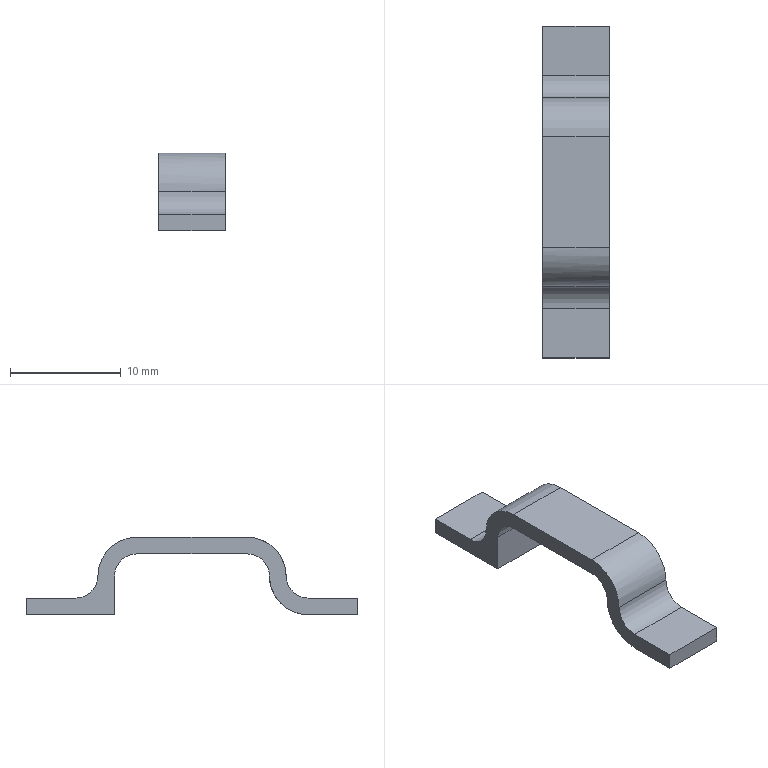Part | NX | features BREP 1 | 1 solid | 18 faces | box 6 x 30 x 7 mm | volume 342.282 mm3 | plane 11 | cylinder 7 | commonest cylinder face diameters 4 x4 7 x3
STEP:
#1=CARTESIAN_POINT('',(41.,114.5,3.5));
#2=VERTEX_POINT('',#1);
#3=CARTESIAN_POINT('',(47.,114.5,3.5));
#4=VERTEX_POINT('',#3);
#5=CARTESIAN_POINT('',(0.,114.5,3.5));
#6=DIRECTION('',(1.,0.,0.));
#7=VECTOR('',#6,1000.);
#8=LINE('',#5,#7);
#9=EDGE_CURVE('',#2,#4,#8,.T.);
#10=ORIENTED_EDGE('',*,*,#9,.F.);
#11=CARTESIAN_POINT('',(41.,111.,7.));
#12=VERTEX_POINT('',#11);
#13=CARTESIAN_POINT('',(41.,111.,3.5));
#14=DIRECTION('',(-1.,0.,0.));
#15=DIRECTION('',(0.,0.,-1.));
#16=AXIS2_PLACEMENT_3D('',#13,#14,#15);
#17=CIRCLE('',#16,3.5);
#18=EDGE_CURVE('',#12,#2,#17,.T.);
#19=ORIENTED_EDGE('',*,*,#18,.F.);
#20=CARTESIAN_POINT('',(47.,111.,7.));
#21=VERTEX_POINT('',#20);
#22=CARTESIAN_POINT('',(0.,111.,7.));
#23=DIRECTION('',(1.,0.,0.));
#24=VECTOR('',#23,1000.);
#25=LINE('',#22,#24);
#26=EDGE_CURVE('',#12,#21,#25,.T.);
#27=ORIENTED_EDGE('',*,*,#26,.T.);
#28=CARTESIAN_POINT('',(47.,111.,3.5));
#29=DIRECTION('',(1.,0.,0.));
#30=DIRECTION('',(0.,0.,-1.));
#31=AXIS2_PLACEMENT_3D('',#28,#29,#30);
#32=CIRCLE('',#31,3.5);
#33=EDGE_CURVE('',#4,#21,#32,.T.);
#34=ORIENTED_EDGE('',*,*,#33,.F.);
#35=EDGE_LOOP('',(#10,#19,#27,#34));
#36=FACE_BOUND('',#35,.T.);
#37=CARTESIAN_POINT('',(0.,111.,3.5));
#38=DIRECTION('',(1.,0.,0.));
#39=DIRECTION('',(0.,1.,0.));
#40=AXIS2_PLACEMENT_3D('',#37,#38,#39);
#41=CYLINDRICAL_SURFACE('',#40,3.5);
#42=ADVANCED_FACE('',(#36),#41,.T.);
#43=ORIENTED_EDGE('',*,*,#9,.T.);
#44=CARTESIAN_POINT('',(47.,116.5,1.5));
#45=VERTEX_POINT('',#44);
#46=CARTESIAN_POINT('',(47.,116.5,3.5));
#47=DIRECTION('',(-1.,0.,0.));
#48=DIRECTION('',(0.,0.,-1.));
#49=AXIS2_PLACEMENT_3D('',#46,#47,#48);
#50=CIRCLE('',#49,2.);
#51=EDGE_CURVE('',#45,#4,#50,.T.);
#52=ORIENTED_EDGE('',*,*,#51,.F.);
#53=CARTESIAN_POINT('',(41.,116.5,1.5));
#54=VERTEX_POINT('',#53);
#55=CARTESIAN_POINT('',(0.,116.5,1.5));
#56=DIRECTION('',(-1.,0.,0.));
#57=VECTOR('',#56,1000.);
#58=LINE('',#55,#57);
#59=EDGE_CURVE('',#45,#54,#58,.T.);
#60=ORIENTED_EDGE('',*,*,#59,.T.);
#61=CARTESIAN_POINT('',(41.,116.5,3.5));
#62=DIRECTION('',(1.,0.,0.));
#63=DIRECTION('',(0.,0.,-1.));
#64=AXIS2_PLACEMENT_3D('',#61,#62,#63);
#65=CIRCLE('',#64,2.);
#66=EDGE_CURVE('',#2,#54,#65,.T.);
#67=ORIENTED_EDGE('',*,*,#66,.F.);
#68=EDGE_LOOP('',(#43,#52,#60,#67));
#69=FACE_BOUND('',#68,.T.);
#70=CARTESIAN_POINT('',(0.,116.5,3.5));
#71=DIRECTION('',(1.,0.,0.));
#72=DIRECTION('',(0.,-1.,0.));
#73=AXIS2_PLACEMENT_3D('',#70,#71,#72);
#74=CYLINDRICAL_SURFACE('',#73,2.);
#75=ADVANCED_FACE('',(#69),#74,.F.);
#76=CARTESIAN_POINT('',(41.,97.5,3.5));
#77=VERTEX_POINT('',#76);
#78=CARTESIAN_POINT('',(41.,101.,7.));
#79=VERTEX_POINT('',#78);
#80=CARTESIAN_POINT('',(41.,97.5,3.5));
#81=CARTESIAN_POINT('',(41.,97.5,3.867));
#82=CARTESIAN_POINT('',(41.,97.548,4.233));
#83=CARTESIAN_POINT('',(41.,97.644,4.591));
#84=CARTESIAN_POINT('',(41.,97.928,5.274));
#85=CARTESIAN_POINT('',(41.,98.377,5.861));
#86=CARTESIAN_POINT('',(41.,98.64,6.124));
#87=CARTESIAN_POINT('',(41.,99.227,6.573));
#88=CARTESIAN_POINT('',(41.,99.909,6.856));
#89=CARTESIAN_POINT('',(41.,100.267,6.952));
#90=CARTESIAN_POINT('',(41.,100.634,7.));
#91=CARTESIAN_POINT('',(41.,101.,7.));
#92=B_SPLINE_CURVE_WITH_KNOTS('',5,(#80,#81,#82,#83,#84,#85,#86,#87,#88,#89,#90,#91),.UNSPECIFIED.,.F.,.F.,(6,3,3,6),(0.,0.3334,0.6668,1.),.UNSPECIFIED.);
#93=EDGE_CURVE('',#77,#79,#92,.T.);
#94=ORIENTED_EDGE('',*,*,#93,.T.);
#95=CARTESIAN_POINT('',(41.,106.,7.));
#96=DIRECTION('',(0.,1.,0.));
#97=VECTOR('',#96,1000.);
#98=LINE('',#95,#97);
#99=EDGE_CURVE('',#79,#12,#98,.T.);
#100=ORIENTED_EDGE('',*,*,#99,.T.);
#101=ORIENTED_EDGE('',*,*,#18,.T.);
#102=ORIENTED_EDGE('',*,*,#66,.T.);
#103=CARTESIAN_POINT('',(41.,121.,1.5));
#104=VERTEX_POINT('',#103);
#105=CARTESIAN_POINT('',(41.,118.75,1.5));
#106=DIRECTION('',(0.,1.,0.));
#107=VECTOR('',#106,1000.);
#108=LINE('',#105,#107);
#109=EDGE_CURVE('',#54,#104,#108,.T.);
#110=ORIENTED_EDGE('',*,*,#109,.T.);
#111=CARTESIAN_POINT('',(41.,121.,0.));
#112=VERTEX_POINT('',#111);
#113=CARTESIAN_POINT('',(41.,121.,0.75));
#114=DIRECTION('',(0.,0.,1.));
#115=VECTOR('',#114,1000.);
#116=LINE('',#113,#115);
#117=EDGE_CURVE('',#112,#104,#116,.T.);
#118=ORIENTED_EDGE('',*,*,#117,.F.);
#119=CARTESIAN_POINT('',(41.,113.,0.));
#120=VERTEX_POINT('',#119);
#121=CARTESIAN_POINT('',(41.,117.,0.));
#122=DIRECTION('',(0.,1.,0.));
#123=VECTOR('',#122,1000.);
#124=LINE('',#121,#123);
#125=EDGE_CURVE('',#120,#112,#124,.T.);
#126=ORIENTED_EDGE('',*,*,#125,.F.);
#127=CARTESIAN_POINT('',(41.,113.,3.5));
#128=VERTEX_POINT('',#127);
#129=CARTESIAN_POINT('',(41.,113.,1.75));
#130=DIRECTION('',(0.,0.,1.));
#131=VECTOR('',#130,1000.);
#132=LINE('',#129,#131);
#133=EDGE_CURVE('',#120,#128,#132,.T.);
#134=ORIENTED_EDGE('',*,*,#133,.T.);
#135=CARTESIAN_POINT('',(41.,111.,5.5));
#136=VERTEX_POINT('',#135);
#137=CARTESIAN_POINT('',(41.,111.,3.5));
#138=DIRECTION('',(1.,0.,0.));
#139=DIRECTION('',(0.,0.,-1.));
#140=AXIS2_PLACEMENT_3D('',#137,#138,#139);
#141=CIRCLE('',#140,2.);
#142=EDGE_CURVE('',#128,#136,#141,.T.);
#143=ORIENTED_EDGE('',*,*,#142,.T.);
#144=CARTESIAN_POINT('',(41.,101.,5.5));
#145=VERTEX_POINT('',#144);
#146=CARTESIAN_POINT('',(41.,106.,5.5));
#147=DIRECTION('',(0.,1.,0.));
#148=VECTOR('',#147,1000.);
#149=LINE('',#146,#148);
#150=EDGE_CURVE('',#145,#136,#149,.T.);
#151=ORIENTED_EDGE('',*,*,#150,.F.);
#152=CARTESIAN_POINT('',(41.,99.,3.5));
#153=VERTEX_POINT('',#152);
#154=CARTESIAN_POINT('',(41.,101.,3.5));
#155=DIRECTION('',(1.,0.,0.));
#156=DIRECTION('',(0.,0.,-1.));
#157=AXIS2_PLACEMENT_3D('',#154,#155,#156);
#158=CIRCLE('',#157,2.);
#159=EDGE_CURVE('',#145,#153,#158,.T.);
#160=ORIENTED_EDGE('',*,*,#159,.T.);
#161=CARTESIAN_POINT('',(41.,95.5,0.));
#162=VERTEX_POINT('',#161);
#163=CARTESIAN_POINT('',(41.,99.,3.5));
#164=CARTESIAN_POINT('',(41.,99.,3.133));
#165=CARTESIAN_POINT('',(41.,98.952,2.767));
#166=CARTESIAN_POINT('',(41.,98.856,2.409));
#167=CARTESIAN_POINT('',(41.,98.572,1.726));
#168=CARTESIAN_POINT('',(41.,98.123,1.139));
#169=CARTESIAN_POINT('',(41.,97.86,0.8765));
#170=CARTESIAN_POINT('',(41.,97.273,0.4271));
#171=CARTESIAN_POINT('',(41.,96.591,0.1438));
#172=CARTESIAN_POINT('',(41.,96.233,0.04793));
#173=CARTESIAN_POINT('',(41.,95.866,0.));
#174=CARTESIAN_POINT('',(41.,95.5,0.));
#175=B_SPLINE_CURVE_WITH_KNOTS('',5,(#163,#164,#165,#166,#167,#168,#169,#170,#171,#172,#173,#174),.UNSPECIFIED.,.F.,.F.,(6,3,3,6),(0.,0.3334,0.6668,1.),.UNSPECIFIED.);
#176=EDGE_CURVE('',#153,#162,#175,.T.);
#177=ORIENTED_EDGE('',*,*,#176,.T.);
#178=CARTESIAN_POINT('',(41.,91.,0.));
#179=VERTEX_POINT('',#178);
#180=CARTESIAN_POINT('',(41.,93.25,0.));
#181=DIRECTION('',(0.,1.,0.));
#182=VECTOR('',#181,1000.);
#183=LINE('',#180,#182);
#184=EDGE_CURVE('',#179,#162,#183,.T.);
#185=ORIENTED_EDGE('',*,*,#184,.F.);
#186=CARTESIAN_POINT('',(41.,91.,1.5));
#187=VERTEX_POINT('',#186);
#188=CARTESIAN_POINT('',(41.,91.,0.75));
#189=DIRECTION('',(0.,0.,1.));
#190=VECTOR('',#189,1000.);
#191=LINE('',#188,#190);
#192=EDGE_CURVE('',#179,#187,#191,.T.);
#193=ORIENTED_EDGE('',*,*,#192,.T.);
#194=CARTESIAN_POINT('',(41.,95.5,1.5));
#195=VERTEX_POINT('',#194);
#196=CARTESIAN_POINT('',(41.,93.25,1.5));
#197=DIRECTION('',(0.,1.,0.));
#198=VECTOR('',#197,1000.);
#199=LINE('',#196,#198);
#200=EDGE_CURVE('',#187,#195,#199,.T.);
#201=ORIENTED_EDGE('',*,*,#200,.T.);
#202=CARTESIAN_POINT('',(41.,95.5,3.5));
#203=DIRECTION('',(1.,0.,0.));
#204=DIRECTION('',(0.,0.,-1.));
#205=AXIS2_PLACEMENT_3D('',#202,#203,#204);
#206=CIRCLE('',#205,2.);
#207=EDGE_CURVE('',#195,#77,#206,.T.);
#208=ORIENTED_EDGE('',*,*,#207,.T.);
#209=EDGE_LOOP('',(#94,#100,#101,#102,#110,#118,#126,#134,#143,#151,#160,#177,#185,#193,#201,#208));
#210=FACE_BOUND('',#209,.T.);
#211=CARTESIAN_POINT('',(41.,121.,1.5));
#212=DIRECTION('',(1.,0.,0.));
#213=DIRECTION('',(0.,-1.,0.));
#214=AXIS2_PLACEMENT_3D('',#211,#212,#213);
#215=PLANE('',#214);
#216=ADVANCED_FACE('',(#210),#215,.F.);
#217=CARTESIAN_POINT('',(47.,101.,7.));
#218=VERTEX_POINT('',#217);
#219=CARTESIAN_POINT('',(44.,101.,7.));
#220=DIRECTION('',(-1.,0.,0.));
#221=VECTOR('',#220,1000.);
#222=LINE('',#219,#221);
#223=EDGE_CURVE('',#218,#79,#222,.T.);
#224=ORIENTED_EDGE('',*,*,#223,.F.);
#225=CARTESIAN_POINT('',(47.,106.,7.));
#226=DIRECTION('',(0.,-1.,0.));
#227=VECTOR('',#226,1000.);
#228=LINE('',#225,#227);
#229=EDGE_CURVE('',#21,#218,#228,.T.);
#230=ORIENTED_EDGE('',*,*,#229,.F.);
#231=ORIENTED_EDGE('',*,*,#26,.F.);
#232=ORIENTED_EDGE('',*,*,#99,.F.);
#233=EDGE_LOOP('',(#224,#230,#231,#232));
#234=FACE_BOUND('',#233,.T.);
#235=CARTESIAN_POINT('',(0.,0.,7.));
#236=DIRECTION('',(0.,0.,1.));
#237=DIRECTION('',(-1.,0.,0.));
#238=AXIS2_PLACEMENT_3D('',#235,#236,#237);
#239=PLANE('',#238);
#240=ADVANCED_FACE('',(#234),#239,.T.);
#241=CARTESIAN_POINT('',(47.,97.5,3.5));
#242=VERTEX_POINT('',#241);
#243=CARTESIAN_POINT('',(47.,101.,7.));
#244=CARTESIAN_POINT('',(47.,100.633,7.));
#245=CARTESIAN_POINT('',(47.,100.267,6.952));
#246=CARTESIAN_POINT('',(47.,99.909,6.856));
#247=CARTESIAN_POINT('',(47.,99.226,6.572));
#248=CARTESIAN_POINT('',(47.,98.639,6.123));
#249=CARTESIAN_POINT('',(47.,98.376,5.86));
#250=CARTESIAN_POINT('',(47.,97.927,5.273));
#251=CARTESIAN_POINT('',(47.,97.644,4.591));
#252=CARTESIAN_POINT('',(47.,97.548,4.233));
#253=CARTESIAN_POINT('',(47.,97.5,3.866));
#254=CARTESIAN_POINT('',(47.,97.5,3.5));
#255=B_SPLINE_CURVE_WITH_KNOTS('',5,(#243,#244,#245,#246,#247,#248,#249,#250,#251,#252,#253,#254),.UNSPECIFIED.,.F.,.F.,(6,3,3,6),(0.,0.3334,0.6668,1.),.UNSPECIFIED.);
#256=EDGE_CURVE('',#218,#242,#255,.T.);
#257=ORIENTED_EDGE('',*,*,#256,.T.);
#258=CARTESIAN_POINT('',(47.,95.5,1.5));
#259=VERTEX_POINT('',#258);
#260=CARTESIAN_POINT('',(47.,95.5,3.5));
#261=DIRECTION('',(-1.,0.,0.));
#262=DIRECTION('',(0.,0.,1.));
#263=AXIS2_PLACEMENT_3D('',#260,#261,#262);
#264=CIRCLE('',#263,2.);
#265=EDGE_CURVE('',#242,#259,#264,.T.);
#266=ORIENTED_EDGE('',*,*,#265,.T.);
#267=CARTESIAN_POINT('',(47.,91.,1.5));
#268=VERTEX_POINT('',#267);
#269=CARTESIAN_POINT('',(47.,93.25,1.5));
#270=DIRECTION('',(0.,-1.,0.));
#271=VECTOR('',#270,1000.);
#272=LINE('',#269,#271);
#273=EDGE_CURVE('',#259,#268,#272,.T.);
#274=ORIENTED_EDGE('',*,*,#273,.T.);
#275=CARTESIAN_POINT('',(47.,91.,0.));
#276=VERTEX_POINT('',#275);
#277=CARTESIAN_POINT('',(47.,91.,0.75));
#278=DIRECTION('',(0.,0.,1.));
#279=VECTOR('',#278,1000.);
#280=LINE('',#277,#279);
#281=EDGE_CURVE('',#276,#268,#280,.T.);
#282=ORIENTED_EDGE('',*,*,#281,.F.);
#283=CARTESIAN_POINT('',(47.,95.5,0.));
#284=VERTEX_POINT('',#283);
#285=CARTESIAN_POINT('',(47.,93.25,0.));
#286=DIRECTION('',(0.,-1.,0.));
#287=VECTOR('',#286,1000.);
#288=LINE('',#285,#287);
#289=EDGE_CURVE('',#284,#276,#288,.T.);
#290=ORIENTED_EDGE('',*,*,#289,.F.);
#291=CARTESIAN_POINT('',(47.,99.,3.5));
#292=VERTEX_POINT('',#291);
#293=CARTESIAN_POINT('',(47.,95.5,0.));
#294=CARTESIAN_POINT('',(47.,95.867,0.));
#295=CARTESIAN_POINT('',(47.,96.233,0.048));
#296=CARTESIAN_POINT('',(47.,96.591,0.144));
#297=CARTESIAN_POINT('',(47.,97.274,0.4276));
#298=CARTESIAN_POINT('',(47.,97.861,0.8773));
#299=CARTESIAN_POINT('',(47.,98.124,1.14));
#300=CARTESIAN_POINT('',(47.,98.573,1.727));
#301=CARTESIAN_POINT('',(47.,98.856,2.409));
#302=CARTESIAN_POINT('',(47.,98.952,2.767));
#303=CARTESIAN_POINT('',(47.,99.,3.134));
#304=CARTESIAN_POINT('',(47.,99.,3.5));
#305=B_SPLINE_CURVE_WITH_KNOTS('',5,(#293,#294,#295,#296,#297,#298,#299,#300,#301,#302,#303,#304),.UNSPECIFIED.,.F.,.F.,(6,3,3,6),(0.,0.3334,0.6668,1.),.UNSPECIFIED.);
#306=EDGE_CURVE('',#284,#292,#305,.T.);
#307=ORIENTED_EDGE('',*,*,#306,.T.);
#308=CARTESIAN_POINT('',(47.,101.,5.5));
#309=VERTEX_POINT('',#308);
#310=CARTESIAN_POINT('',(47.,101.,3.5));
#311=DIRECTION('',(-1.,0.,0.));
#312=DIRECTION('',(0.,0.,1.));
#313=AXIS2_PLACEMENT_3D('',#310,#311,#312);
#314=CIRCLE('',#313,2.);
#315=EDGE_CURVE('',#292,#309,#314,.T.);
#316=ORIENTED_EDGE('',*,*,#315,.T.);
#317=CARTESIAN_POINT('',(47.,111.,5.5));
#318=VERTEX_POINT('',#317);
#319=CARTESIAN_POINT('',(47.,106.,5.5));
#320=DIRECTION('',(0.,-1.,0.));
#321=VECTOR('',#320,1000.);
#322=LINE('',#319,#321);
#323=EDGE_CURVE('',#318,#309,#322,.T.);
#324=ORIENTED_EDGE('',*,*,#323,.F.);
#325=CARTESIAN_POINT('',(47.,113.,3.5));
#326=VERTEX_POINT('',#325);
#327=CARTESIAN_POINT('',(47.,111.,3.5));
#328=DIRECTION('',(-1.,0.,0.));
#329=DIRECTION('',(0.,0.,1.));
#330=AXIS2_PLACEMENT_3D('',#327,#328,#329);
#331=CIRCLE('',#330,2.);
#332=EDGE_CURVE('',#318,#326,#331,.T.);
#333=ORIENTED_EDGE('',*,*,#332,.T.);
#334=CARTESIAN_POINT('',(47.,113.,0.));
#335=VERTEX_POINT('',#334);
#336=CARTESIAN_POINT('',(47.,113.,1.75));
#337=DIRECTION('',(0.,0.,1.));
#338=VECTOR('',#337,1000.);
#339=LINE('',#336,#338);
#340=EDGE_CURVE('',#335,#326,#339,.T.);
#341=ORIENTED_EDGE('',*,*,#340,.F.);
#342=CARTESIAN_POINT('',(47.,121.,0.));
#343=VERTEX_POINT('',#342);
#344=CARTESIAN_POINT('',(47.,117.,0.));
#345=DIRECTION('',(0.,-1.,0.));
#346=VECTOR('',#345,1000.);
#347=LINE('',#344,#346);
#348=EDGE_CURVE('',#343,#335,#347,.T.);
#349=ORIENTED_EDGE('',*,*,#348,.F.);
#350=CARTESIAN_POINT('',(47.,121.,1.5));
#351=VERTEX_POINT('',#350);
#352=CARTESIAN_POINT('',(47.,121.,0.75));
#353=DIRECTION('',(0.,0.,1.));
#354=VECTOR('',#353,1000.);
#355=LINE('',#352,#354);
#356=EDGE_CURVE('',#343,#351,#355,.T.);
#357=ORIENTED_EDGE('',*,*,#356,.T.);
#358=CARTESIAN_POINT('',(47.,118.75,1.5));
#359=DIRECTION('',(0.,-1.,0.));
#360=VECTOR('',#359,1000.);
#361=LINE('',#358,#360);
#362=EDGE_CURVE('',#351,#45,#361,.T.);
#363=ORIENTED_EDGE('',*,*,#362,.T.);
#364=ORIENTED_EDGE('',*,*,#51,.T.);
#365=ORIENTED_EDGE('',*,*,#33,.T.);
#366=ORIENTED_EDGE('',*,*,#229,.T.);
#367=EDGE_LOOP('',(#257,#266,#274,#282,#290,#307,#316,#324,#333,#341,#349,#357,#363,#364,#365,#366));
#368=FACE_BOUND('',#367,.T.);
#369=CARTESIAN_POINT('',(47.,91.,1.5));
#370=DIRECTION('',(-1.,0.,0.));
#371=DIRECTION('',(0.,0.,-1.));
#372=AXIS2_PLACEMENT_3D('',#369,#370,#371);
#373=PLANE('',#372);
#374=ADVANCED_FACE('',(#368),#373,.F.);
#375=ORIENTED_EDGE('',*,*,#59,.F.);
#376=ORIENTED_EDGE('',*,*,#362,.F.);
#377=CARTESIAN_POINT('',(44.,121.,1.5));
#378=DIRECTION('',(1.,0.,0.));
#379=VECTOR('',#378,1000.);
#380=LINE('',#377,#379);
#381=EDGE_CURVE('',#104,#351,#380,.T.);
#382=ORIENTED_EDGE('',*,*,#381,.F.);
#383=ORIENTED_EDGE('',*,*,#109,.F.);
#384=EDGE_LOOP('',(#375,#376,#382,#383));
#385=FACE_BOUND('',#384,.T.);
#386=CARTESIAN_POINT('',(0.,0.,1.5));
#387=DIRECTION('',(0.,0.,1.));
#388=DIRECTION('',(-1.,0.,0.));
#389=AXIS2_PLACEMENT_3D('',#386,#387,#388);
#390=PLANE('',#389);
#391=ADVANCED_FACE('',(#385),#390,.T.);
#392=CARTESIAN_POINT('',(0.,97.5,3.5));
#393=DIRECTION('',(-1.,0.,0.));
#394=VECTOR('',#393,1000.);
#395=LINE('',#392,#394);
#396=EDGE_CURVE('',#242,#77,#395,.T.);
#397=ORIENTED_EDGE('',*,*,#396,.F.);
#398=ORIENTED_EDGE('',*,*,#256,.F.);
#399=ORIENTED_EDGE('',*,*,#223,.T.);
#400=ORIENTED_EDGE('',*,*,#93,.F.);
#401=EDGE_LOOP('',(#397,#398,#399,#400));
#402=FACE_BOUND('',#401,.T.);
#403=CARTESIAN_POINT('',(0.,101.,3.5));
#404=DIRECTION('',(-1.,0.,0.));
#405=DIRECTION('',(0.,-1.,0.));
#406=AXIS2_PLACEMENT_3D('',#403,#404,#405);
#407=CYLINDRICAL_SURFACE('',#406,3.5);
#408=ADVANCED_FACE('',(#402),#407,.T.);
#409=ORIENTED_EDGE('',*,*,#117,.T.);
#410=ORIENTED_EDGE('',*,*,#381,.T.);
#411=ORIENTED_EDGE('',*,*,#356,.F.);
#412=CARTESIAN_POINT('',(44.,121.,0.));
#413=DIRECTION('',(1.,0.,0.));
#414=VECTOR('',#413,1000.);
#415=LINE('',#412,#414);
#416=EDGE_CURVE('',#112,#343,#415,.T.);
#417=ORIENTED_EDGE('',*,*,#416,.F.);
#418=EDGE_LOOP('',(#409,#410,#411,#417));
#419=FACE_BOUND('',#418,.T.);
#420=CARTESIAN_POINT('',(47.,121.,1.5));
#421=DIRECTION('',(0.,-1.,0.));
#422=DIRECTION('',(0.,0.,1.));
#423=AXIS2_PLACEMENT_3D('',#420,#421,#422);
#424=PLANE('',#423);
#425=ADVANCED_FACE('',(#419),#424,.F.);
#426=CARTESIAN_POINT('',(44.,113.,0.));
#427=DIRECTION('',(1.,0.,0.));
#428=VECTOR('',#427,1000.);
#429=LINE('',#426,#428);
#430=EDGE_CURVE('',#120,#335,#429,.T.);
#431=ORIENTED_EDGE('',*,*,#430,.F.);
#432=ORIENTED_EDGE('',*,*,#125,.T.);
#433=ORIENTED_EDGE('',*,*,#416,.T.);
#434=ORIENTED_EDGE('',*,*,#348,.T.);
#435=EDGE_LOOP('',(#431,#432,#433,#434));
#436=FACE_BOUND('',#435,.T.);
#437=CARTESIAN_POINT('',(0.,0.,0.));
#438=DIRECTION('',(0.,0.,1.));
#439=DIRECTION('',(-1.,0.,0.));
#440=AXIS2_PLACEMENT_3D('',#437,#438,#439);
#441=PLANE('',#440);
#442=ADVANCED_FACE('',(#436),#441,.F.);
#443=CARTESIAN_POINT('',(44.,113.,3.5));
#444=DIRECTION('',(1.,0.,0.));
#445=VECTOR('',#444,1000.);
#446=LINE('',#443,#445);
#447=EDGE_CURVE('',#128,#326,#446,.T.);
#448=ORIENTED_EDGE('',*,*,#447,.F.);
#449=ORIENTED_EDGE('',*,*,#133,.F.);
#450=ORIENTED_EDGE('',*,*,#430,.T.);
#451=ORIENTED_EDGE('',*,*,#340,.T.);
#452=EDGE_LOOP('',(#448,#449,#450,#451));
#453=FACE_BOUND('',#452,.T.);
#454=CARTESIAN_POINT('',(54.,113.,7.));
#455=DIRECTION('',(0.,-1.,0.));
#456=DIRECTION('',(0.,0.,1.));
#457=AXIS2_PLACEMENT_3D('',#454,#455,#456);
#458=PLANE('',#457);
#459=ADVANCED_FACE('',(#453),#458,.T.);
#460=CARTESIAN_POINT('',(54.,111.,5.5));
#461=DIRECTION('',(-1.,0.,0.));
#462=VECTOR('',#461,1000.);
#463=LINE('',#460,#462);
#464=EDGE_CURVE('',#318,#136,#463,.T.);
#465=ORIENTED_EDGE('',*,*,#464,.T.);
#466=ORIENTED_EDGE('',*,*,#142,.F.);
#467=ORIENTED_EDGE('',*,*,#447,.T.);
#468=ORIENTED_EDGE('',*,*,#332,.F.);
#469=EDGE_LOOP('',(#465,#466,#467,#468));
#470=FACE_BOUND('',#469,.T.);
#471=CARTESIAN_POINT('',(54.,111.,3.5));
#472=DIRECTION('',(-1.,0.,0.));
#473=DIRECTION('',(0.,-1.,0.));
#474=AXIS2_PLACEMENT_3D('',#471,#472,#473);
#475=CYLINDRICAL_SURFACE('',#474,2.);
#476=ADVANCED_FACE('',(#470),#475,.F.);
#477=CARTESIAN_POINT('',(44.,101.,5.5));
#478=DIRECTION('',(1.,0.,0.));
#479=VECTOR('',#478,1000.);
#480=LINE('',#477,#479);
#481=EDGE_CURVE('',#145,#309,#480,.T.);
#482=ORIENTED_EDGE('',*,*,#481,.F.);
#483=ORIENTED_EDGE('',*,*,#150,.T.);
#484=ORIENTED_EDGE('',*,*,#464,.F.);
#485=ORIENTED_EDGE('',*,*,#323,.T.);
#486=EDGE_LOOP('',(#482,#483,#484,#485));
#487=FACE_BOUND('',#486,.T.);
#488=CARTESIAN_POINT('',(0.,0.,5.5));
#489=DIRECTION('',(0.,0.,1.));
#490=DIRECTION('',(-1.,0.,0.));
#491=AXIS2_PLACEMENT_3D('',#488,#489,#490);
#492=PLANE('',#491);
#493=ADVANCED_FACE('',(#487),#492,.F.);
#494=ORIENTED_EDGE('',*,*,#481,.T.);
#495=ORIENTED_EDGE('',*,*,#315,.F.);
#496=CARTESIAN_POINT('',(36.5,99.,3.5));
#497=DIRECTION('',(1.,0.,0.));
#498=VECTOR('',#497,1000.);
#499=LINE('',#496,#498);
#500=EDGE_CURVE('',#153,#292,#499,.T.);
#501=ORIENTED_EDGE('',*,*,#500,.F.);
#502=ORIENTED_EDGE('',*,*,#159,.F.);
#503=EDGE_LOOP('',(#494,#495,#501,#502));
#504=FACE_BOUND('',#503,.T.);
#505=CARTESIAN_POINT('',(36.5,101.,3.5));
#506=DIRECTION('',(1.,0.,0.));
#507=DIRECTION('',(0.,1.,0.));
#508=AXIS2_PLACEMENT_3D('',#505,#506,#507);
#509=CYLINDRICAL_SURFACE('',#508,2.);
#510=ADVANCED_FACE('',(#504),#509,.F.);
#511=ORIENTED_EDGE('',*,*,#500,.T.);
#512=ORIENTED_EDGE('',*,*,#306,.F.);
#513=CARTESIAN_POINT('',(0.,95.5,0.));
#514=DIRECTION('',(-1.,0.,0.));
#515=VECTOR('',#514,1000.);
#516=LINE('',#513,#515);
#517=EDGE_CURVE('',#284,#162,#516,.T.);
#518=ORIENTED_EDGE('',*,*,#517,.T.);
#519=ORIENTED_EDGE('',*,*,#176,.F.);
#520=EDGE_LOOP('',(#511,#512,#518,#519));
#521=FACE_BOUND('',#520,.T.);
#522=CARTESIAN_POINT('',(0.,95.5,3.5));
#523=DIRECTION('',(-1.,0.,0.));
#524=DIRECTION('',(0.,1.,0.));
#525=AXIS2_PLACEMENT_3D('',#522,#523,#524);
#526=CYLINDRICAL_SURFACE('',#525,3.5);
#527=ADVANCED_FACE('',(#521),#526,.T.);
#528=ORIENTED_EDGE('',*,*,#517,.F.);
#529=ORIENTED_EDGE('',*,*,#289,.T.);
#530=CARTESIAN_POINT('',(44.,91.,0.));
#531=DIRECTION('',(-1.,0.,0.));
#532=VECTOR('',#531,1000.);
#533=LINE('',#530,#532);
#534=EDGE_CURVE('',#276,#179,#533,.T.);
#535=ORIENTED_EDGE('',*,*,#534,.T.);
#536=ORIENTED_EDGE('',*,*,#184,.T.);
#537=EDGE_LOOP('',(#528,#529,#535,#536));
#538=FACE_BOUND('',#537,.T.);
#539=CARTESIAN_POINT('',(0.,0.,0.));
#540=DIRECTION('',(0.,0.,1.));
#541=DIRECTION('',(-1.,0.,0.));
#542=AXIS2_PLACEMENT_3D('',#539,#540,#541);
#543=PLANE('',#542);
#544=ADVANCED_FACE('',(#538),#543,.F.);
#545=ORIENTED_EDGE('',*,*,#281,.T.);
#546=CARTESIAN_POINT('',(44.,91.,1.5));
#547=DIRECTION('',(-1.,0.,0.));
#548=VECTOR('',#547,1000.);
#549=LINE('',#546,#548);
#550=EDGE_CURVE('',#268,#187,#549,.T.);
#551=ORIENTED_EDGE('',*,*,#550,.T.);
#552=ORIENTED_EDGE('',*,*,#192,.F.);
#553=ORIENTED_EDGE('',*,*,#534,.F.);
#554=EDGE_LOOP('',(#545,#551,#552,#553));
#555=FACE_BOUND('',#554,.T.);
#556=CARTESIAN_POINT('',(41.,91.,1.5));
#557=DIRECTION('',(0.,1.,0.));
#558=DIRECTION('',(-1.,0.,0.));
#559=AXIS2_PLACEMENT_3D('',#556,#557,#558);
#560=PLANE('',#559);
#561=ADVANCED_FACE('',(#555),#560,.F.);
#562=CARTESIAN_POINT('',(44.,95.5,1.5));
#563=DIRECTION('',(1.,0.,0.));
#564=VECTOR('',#563,1000.);
#565=LINE('',#562,#564);
#566=EDGE_CURVE('',#195,#259,#565,.T.);
#567=ORIENTED_EDGE('',*,*,#566,.F.);
#568=ORIENTED_EDGE('',*,*,#200,.F.);
#569=ORIENTED_EDGE('',*,*,#550,.F.);
#570=ORIENTED_EDGE('',*,*,#273,.F.);
#571=EDGE_LOOP('',(#567,#568,#569,#570));
#572=FACE_BOUND('',#571,.T.);
#573=CARTESIAN_POINT('',(0.,0.,1.5));
#574=DIRECTION('',(0.,0.,1.));
#575=DIRECTION('',(-1.,0.,0.));
#576=AXIS2_PLACEMENT_3D('',#573,#574,#575);
#577=PLANE('',#576);
#578=ADVANCED_FACE('',(#572),#577,.T.);
#579=ORIENTED_EDGE('',*,*,#396,.T.);
#580=ORIENTED_EDGE('',*,*,#207,.F.);
#581=ORIENTED_EDGE('',*,*,#566,.T.);
#582=ORIENTED_EDGE('',*,*,#265,.F.);
#583=EDGE_LOOP('',(#579,#580,#581,#582));
#584=FACE_BOUND('',#583,.T.);
#585=CARTESIAN_POINT('',(0.,95.5,3.5));
#586=DIRECTION('',(-1.,0.,0.));
#587=DIRECTION('',(0.,1.,0.));
#588=AXIS2_PLACEMENT_3D('',#585,#586,#587);
#589=CYLINDRICAL_SURFACE('',#588,2.);
#590=ADVANCED_FACE('',(#584),#589,.F.);
#591=CLOSED_SHELL('',(#42,#75,#216,#240,#374,#391,#408,#425,#442,#459,#476,#493,#510,#527,#544,#561,#578,#590));
#592=MANIFOLD_SOLID_BREP('',#591);
#593=(LENGTH_UNIT()NAMED_UNIT(*)SI_UNIT(.MILLI.,.METRE.));
#594=UNCERTAINTY_MEASURE_WITH_UNIT(LENGTH_MEASURE(0.00001),#593,'','');
#595=(NAMED_UNIT(*)PLANE_ANGLE_UNIT()SI_UNIT($,.RADIAN.));
#596=(NAMED_UNIT(*)SI_UNIT($,.STERADIAN.)SOLID_ANGLE_UNIT());
#597=(GEOMETRIC_REPRESENTATION_CONTEXT(3)GLOBAL_UNCERTAINTY_ASSIGNED_CONTEXT((#594))GLOBAL_UNIT_ASSIGNED_CONTEXT((#593,#595,#596))REPRESENTATION_CONTEXT('',''));
#598=ADVANCED_BREP_SHAPE_REPRESENTATION('',(#592),#597);